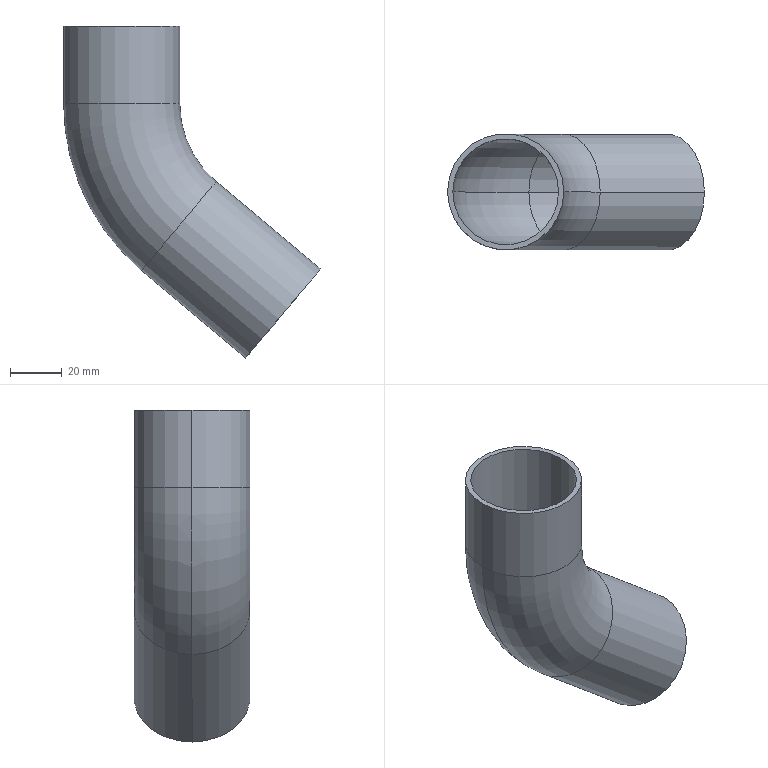Part | SolidWorks | features Shell 1, Sweep 1 | 1 solid | 14 faces | box 99.465 x 45 x 128.591 mm | volume 36956 mm3 | cylinder 8 | torus 4 | plane 2 | commonest cylinder face diameters 41 x4 45 x4
STEP:
#1=CARTESIAN_POINT('',(20.5,0.,-29.999));
#2=VERTEX_POINT('',#1);
#3=CARTESIAN_POINT('',(-20.5,0.,-29.999));
#4=VERTEX_POINT('',#3);
#5=CARTESIAN_POINT('',(0.,0.,-29.999));
#6=DIRECTION('',(0.,0.,1.));
#7=DIRECTION('',(1.,0.,0.));
#8=AXIS2_PLACEMENT_3D('',#5,#6,#7);
#9=CIRCLE('',#8,20.5);
#10=EDGE_CURVE('',#2,#4,#9,.T.);
#11=ORIENTED_EDGE('',*,*,#10,.T.);
#12=CARTESIAN_POINT('',(8.97,0.,-93.198));
#13=VERTEX_POINT('',#12);
#14=CARTESIAN_POINT('',(62.,0.,-29.999));
#15=DIRECTION('',(0.,-1.,0.));
#16=DIRECTION('',(0.,0.,-1.));
#17=AXIS2_PLACEMENT_3D('',#14,#15,#16);
#18=CIRCLE('',#17,82.5);
#19=EDGE_CURVE('',#4,#13,#18,.T.);
#20=ORIENTED_EDGE('',*,*,#19,.T.);
#21=CARTESIAN_POINT('',(35.324,0.,-61.79));
#22=VERTEX_POINT('',#21);
#23=CARTESIAN_POINT('',(22.147,0.,-77.494));
#24=DIRECTION('',(-0.766,0.,0.6428));
#25=DIRECTION('',(0.6428,0.,0.766));
#26=AXIS2_PLACEMENT_3D('',#23,#24,#25);
#27=CIRCLE('',#26,20.5);
#28=EDGE_CURVE('',#22,#13,#27,.T.);
#29=ORIENTED_EDGE('',*,*,#28,.F.);
#30=CARTESIAN_POINT('',(62.,0.,-29.999));
#31=DIRECTION('',(0.,-1.,0.));
#32=DIRECTION('',(0.,0.,-1.));
#33=AXIS2_PLACEMENT_3D('',#30,#31,#32);
#34=CIRCLE('',#33,41.5);
#35=EDGE_CURVE('',#2,#22,#34,.T.);
#36=ORIENTED_EDGE('',*,*,#35,.F.);
#37=EDGE_LOOP('',(#11,#20,#29,#36));
#38=FACE_OUTER_BOUND('',#37,.T.);
#39=CARTESIAN_POINT('',(62.,0.,-29.999));
#40=DIRECTION('',(0.,-1.,0.));
#41=DIRECTION('',(0.,0.,-1.));
#42=AXIS2_PLACEMENT_3D('',#39,#40,#41);
#43=TOROIDAL_SURFACE('',#42,62.,20.5);
#44=ADVANCED_FACE('',(#38),#43,.F.);
#45=CARTESIAN_POINT('',(-22.5,0.,-29.999));
#46=VERTEX_POINT('',#45);
#47=CARTESIAN_POINT('',(22.5,0.,-29.999));
#48=VERTEX_POINT('',#47);
#49=CARTESIAN_POINT('',(0.,0.,-29.999));
#50=DIRECTION('',(0.,0.,1.));
#51=DIRECTION('',(1.,0.,0.));
#52=AXIS2_PLACEMENT_3D('',#49,#50,#51);
#53=CIRCLE('',#52,22.5);
#54=EDGE_CURVE('',#46,#48,#53,.T.);
#55=ORIENTED_EDGE('',*,*,#54,.F.);
#56=CARTESIAN_POINT('',(7.684,0.,-94.73));
#57=VERTEX_POINT('',#56);
#58=CARTESIAN_POINT('',(62.,0.,-29.999));
#59=DIRECTION('',(0.,-1.,0.));
#60=DIRECTION('',(0.,0.,-1.));
#61=AXIS2_PLACEMENT_3D('',#58,#59,#60);
#62=CIRCLE('',#61,84.5);
#63=EDGE_CURVE('',#46,#57,#62,.T.);
#64=ORIENTED_EDGE('',*,*,#63,.T.);
#65=CARTESIAN_POINT('',(36.61,0.,-60.258));
#66=VERTEX_POINT('',#65);
#67=CARTESIAN_POINT('',(22.147,0.,-77.494));
#68=DIRECTION('',(-0.766,0.,0.6428));
#69=DIRECTION('',(0.6428,0.,0.766));
#70=AXIS2_PLACEMENT_3D('',#67,#68,#69);
#71=CIRCLE('',#70,22.5);
#72=EDGE_CURVE('',#57,#66,#71,.T.);
#73=ORIENTED_EDGE('',*,*,#72,.T.);
#74=CARTESIAN_POINT('',(62.,0.,-29.999));
#75=DIRECTION('',(0.,-1.,0.));
#76=DIRECTION('',(0.,0.,-1.));
#77=AXIS2_PLACEMENT_3D('',#74,#75,#76);
#78=CIRCLE('',#77,39.5);
#79=EDGE_CURVE('',#48,#66,#78,.T.);
#80=ORIENTED_EDGE('',*,*,#79,.F.);
#81=EDGE_LOOP('',(#55,#64,#73,#80));
#82=FACE_OUTER_BOUND('',#81,.T.);
#83=CARTESIAN_POINT('',(62.,0.,-29.999));
#84=DIRECTION('',(0.,-1.,0.));
#85=DIRECTION('',(0.,0.,-1.));
#86=AXIS2_PLACEMENT_3D('',#83,#84,#85);
#87=TOROIDAL_SURFACE('',#86,62.,22.5);
#88=ADVANCED_FACE('',(#82),#87,.T.);
#89=CARTESIAN_POINT('',(0.,0.,-29.999));
#90=DIRECTION('',(0.,0.,1.));
#91=DIRECTION('',(1.,0.,0.));
#92=AXIS2_PLACEMENT_3D('',#89,#90,#91);
#93=CIRCLE('',#92,20.5);
#94=EDGE_CURVE('',#4,#2,#93,.T.);
#95=ORIENTED_EDGE('',*,*,#94,.F.);
#96=CARTESIAN_POINT('',(-20.5,0.,0.));
#97=VERTEX_POINT('',#96);
#98=CARTESIAN_POINT('',(-20.5,0.,-29.999));
#99=DIRECTION('',(0.,0.,1.));
#100=VECTOR('',#99,1000.);
#101=LINE('',#98,#100);
#102=EDGE_CURVE('',#4,#97,#101,.T.);
#103=ORIENTED_EDGE('',*,*,#102,.T.);
#104=CARTESIAN_POINT('',(20.5,0.,0.));
#105=VERTEX_POINT('',#104);
#106=CARTESIAN_POINT('',(0.,0.,0.));
#107=DIRECTION('',(0.,0.,1.));
#108=DIRECTION('',(1.,0.,0.));
#109=AXIS2_PLACEMENT_3D('',#106,#107,#108);
#110=CIRCLE('',#109,20.5);
#111=EDGE_CURVE('',#97,#105,#110,.T.);
#112=ORIENTED_EDGE('',*,*,#111,.T.);
#113=CARTESIAN_POINT('',(20.5,0.,-29.999));
#114=DIRECTION('',(0.,0.,1.));
#115=VECTOR('',#114,1000.);
#116=LINE('',#113,#115);
#117=EDGE_CURVE('',#2,#105,#116,.T.);
#118=ORIENTED_EDGE('',*,*,#117,.F.);
#119=EDGE_LOOP('',(#95,#103,#112,#118));
#120=FACE_OUTER_BOUND('',#119,.T.);
#121=CARTESIAN_POINT('',(0.,0.,-29.999));
#122=DIRECTION('',(0.,0.,1.));
#123=DIRECTION('',(1.,0.,0.));
#124=AXIS2_PLACEMENT_3D('',#121,#122,#123);
#125=CYLINDRICAL_SURFACE('',#124,20.5);
#126=ADVANCED_FACE('',(#120),#125,.F.);
#127=CARTESIAN_POINT('',(22.147,0.,-77.494));
#128=DIRECTION('',(-0.766,0.,0.6428));
#129=DIRECTION('',(0.6428,0.,0.766));
#130=AXIS2_PLACEMENT_3D('',#127,#128,#129);
#131=CIRCLE('',#130,20.5);
#132=EDGE_CURVE('',#13,#22,#131,.T.);
#133=ORIENTED_EDGE('',*,*,#132,.T.);
#134=CARTESIAN_POINT('',(75.679,0.,-95.652));
#135=VERTEX_POINT('',#134);
#136=CARTESIAN_POINT('',(35.324,0.,-61.79));
#137=DIRECTION('',(0.766,0.,-0.6428));
#138=VECTOR('',#137,1000.);
#139=LINE('',#136,#138);
#140=EDGE_CURVE('',#22,#135,#139,.T.);
#141=ORIENTED_EDGE('',*,*,#140,.T.);
#142=CARTESIAN_POINT('',(49.325,0.,-127.059));
#143=VERTEX_POINT('',#142);
#144=CARTESIAN_POINT('',(62.502,0.,-111.355));
#145=DIRECTION('',(-0.766,0.,0.6428));
#146=DIRECTION('',(0.6428,0.,0.766));
#147=AXIS2_PLACEMENT_3D('',#144,#145,#146);
#148=CIRCLE('',#147,20.5);
#149=EDGE_CURVE('',#143,#135,#148,.T.);
#150=ORIENTED_EDGE('',*,*,#149,.F.);
#151=CARTESIAN_POINT('',(8.97,0.,-93.198));
#152=DIRECTION('',(0.766,0.,-0.6428));
#153=VECTOR('',#152,1000.);
#154=LINE('',#151,#153);
#155=EDGE_CURVE('',#13,#143,#154,.T.);
#156=ORIENTED_EDGE('',*,*,#155,.F.);
#157=EDGE_LOOP('',(#133,#141,#150,#156));
#158=FACE_OUTER_BOUND('',#157,.T.);
#159=CARTESIAN_POINT('',(22.147,0.,-77.494));
#160=DIRECTION('',(0.766,0.,-0.6428));
#161=DIRECTION('',(-0.6428,0.,-0.766));
#162=AXIS2_PLACEMENT_3D('',#159,#160,#161);
#163=CYLINDRICAL_SURFACE('',#162,20.5);
#164=ADVANCED_FACE('',(#158),#163,.F.);
#165=CARTESIAN_POINT('',(0.,0.,-29.999));
#166=DIRECTION('',(0.,0.,1.));
#167=DIRECTION('',(1.,0.,0.));
#168=AXIS2_PLACEMENT_3D('',#165,#166,#167);
#169=CIRCLE('',#168,22.5);
#170=EDGE_CURVE('',#48,#46,#169,.T.);
#171=ORIENTED_EDGE('',*,*,#170,.T.);
#172=CARTESIAN_POINT('',(-22.5,0.,0.));
#173=VERTEX_POINT('',#172);
#174=CARTESIAN_POINT('',(-22.5,0.,-29.999));
#175=DIRECTION('',(0.,0.,1.));
#176=VECTOR('',#175,1000.);
#177=LINE('',#174,#176);
#178=EDGE_CURVE('',#46,#173,#177,.T.);
#179=ORIENTED_EDGE('',*,*,#178,.T.);
#180=CARTESIAN_POINT('',(22.5,0.,0.));
#181=VERTEX_POINT('',#180);
#182=CARTESIAN_POINT('',(0.,0.,0.));
#183=DIRECTION('',(0.,0.,1.));
#184=DIRECTION('',(1.,0.,0.));
#185=AXIS2_PLACEMENT_3D('',#182,#183,#184);
#186=CIRCLE('',#185,22.5);
#187=EDGE_CURVE('',#181,#173,#186,.T.);
#188=ORIENTED_EDGE('',*,*,#187,.F.);
#189=CARTESIAN_POINT('',(22.5,0.,-29.999));
#190=DIRECTION('',(0.,0.,1.));
#191=VECTOR('',#190,1000.);
#192=LINE('',#189,#191);
#193=EDGE_CURVE('',#48,#181,#192,.T.);
#194=ORIENTED_EDGE('',*,*,#193,.F.);
#195=EDGE_LOOP('',(#171,#179,#188,#194));
#196=FACE_OUTER_BOUND('',#195,.T.);
#197=CARTESIAN_POINT('',(0.,0.,-29.999));
#198=DIRECTION('',(0.,0.,1.));
#199=DIRECTION('',(1.,0.,0.));
#200=AXIS2_PLACEMENT_3D('',#197,#198,#199);
#201=CYLINDRICAL_SURFACE('',#200,22.5);
#202=ADVANCED_FACE('',(#196),#201,.T.);
#203=CARTESIAN_POINT('',(22.147,0.,-77.494));
#204=DIRECTION('',(-0.766,0.,0.6428));
#205=DIRECTION('',(0.6428,0.,0.766));
#206=AXIS2_PLACEMENT_3D('',#203,#204,#205);
#207=CIRCLE('',#206,22.5);
#208=EDGE_CURVE('',#66,#57,#207,.T.);
#209=ORIENTED_EDGE('',*,*,#208,.F.);
#210=CARTESIAN_POINT('',(76.965,0.,-94.119));
#211=VERTEX_POINT('',#210);
#212=CARTESIAN_POINT('',(36.61,0.,-60.258));
#213=DIRECTION('',(0.766,0.,-0.6428));
#214=VECTOR('',#213,1000.);
#215=LINE('',#212,#214);
#216=EDGE_CURVE('',#66,#211,#215,.T.);
#217=ORIENTED_EDGE('',*,*,#216,.T.);
#218=CARTESIAN_POINT('',(48.039,0.,-128.591));
#219=VERTEX_POINT('',#218);
#220=CARTESIAN_POINT('',(62.502,0.,-111.355));
#221=DIRECTION('',(-0.766,0.,0.6428));
#222=DIRECTION('',(0.6428,0.,0.766));
#223=AXIS2_PLACEMENT_3D('',#220,#221,#222);
#224=CIRCLE('',#223,22.5);
#225=EDGE_CURVE('',#211,#219,#224,.T.);
#226=ORIENTED_EDGE('',*,*,#225,.T.);
#227=CARTESIAN_POINT('',(7.684,0.,-94.73));
#228=DIRECTION('',(0.766,0.,-0.6428));
#229=VECTOR('',#228,1000.);
#230=LINE('',#227,#229);
#231=EDGE_CURVE('',#57,#219,#230,.T.);
#232=ORIENTED_EDGE('',*,*,#231,.F.);
#233=EDGE_LOOP('',(#209,#217,#226,#232));
#234=FACE_OUTER_BOUND('',#233,.T.);
#235=CARTESIAN_POINT('',(22.147,0.,-77.494));
#236=DIRECTION('',(0.766,0.,-0.6428));
#237=DIRECTION('',(-0.6428,0.,-0.766));
#238=AXIS2_PLACEMENT_3D('',#235,#236,#237);
#239=CYLINDRICAL_SURFACE('',#238,22.5);
#240=ADVANCED_FACE('',(#234),#239,.T.);
#241=ORIENTED_EDGE('',*,*,#216,.F.);
#242=ORIENTED_EDGE('',*,*,#72,.F.);
#243=ORIENTED_EDGE('',*,*,#231,.T.);
#244=CARTESIAN_POINT('',(62.502,0.,-111.355));
#245=DIRECTION('',(-0.766,0.,0.6428));
#246=DIRECTION('',(0.6428,0.,0.766));
#247=AXIS2_PLACEMENT_3D('',#244,#245,#246);
#248=CIRCLE('',#247,22.5);
#249=EDGE_CURVE('',#219,#211,#248,.T.);
#250=ORIENTED_EDGE('',*,*,#249,.T.);
#251=EDGE_LOOP('',(#241,#242,#243,#250));
#252=FACE_OUTER_BOUND('',#251,.T.);
#253=CARTESIAN_POINT('',(22.147,0.,-77.494));
#254=DIRECTION('',(0.766,0.,-0.6428));
#255=DIRECTION('',(-0.6428,0.,-0.766));
#256=AXIS2_PLACEMENT_3D('',#253,#254,#255);
#257=CYLINDRICAL_SURFACE('',#256,22.5);
#258=ADVANCED_FACE('',(#252),#257,.T.);
#259=ORIENTED_EDGE('',*,*,#63,.F.);
#260=ORIENTED_EDGE('',*,*,#170,.F.);
#261=ORIENTED_EDGE('',*,*,#79,.T.);
#262=ORIENTED_EDGE('',*,*,#208,.T.);
#263=EDGE_LOOP('',(#259,#260,#261,#262));
#264=FACE_OUTER_BOUND('',#263,.T.);
#265=CARTESIAN_POINT('',(62.,0.,-29.999));
#266=DIRECTION('',(0.,-1.,0.));
#267=DIRECTION('',(0.,0.,-1.));
#268=AXIS2_PLACEMENT_3D('',#265,#266,#267);
#269=TOROIDAL_SURFACE('',#268,62.,22.5);
#270=ADVANCED_FACE('',(#264),#269,.T.);
#271=ORIENTED_EDGE('',*,*,#178,.F.);
#272=ORIENTED_EDGE('',*,*,#54,.T.);
#273=ORIENTED_EDGE('',*,*,#193,.T.);
#274=CARTESIAN_POINT('',(0.,0.,0.));
#275=DIRECTION('',(0.,0.,1.));
#276=DIRECTION('',(1.,0.,0.));
#277=AXIS2_PLACEMENT_3D('',#274,#275,#276);
#278=CIRCLE('',#277,22.5);
#279=EDGE_CURVE('',#173,#181,#278,.T.);
#280=ORIENTED_EDGE('',*,*,#279,.F.);
#281=EDGE_LOOP('',(#271,#272,#273,#280));
#282=FACE_OUTER_BOUND('',#281,.T.);
#283=CARTESIAN_POINT('',(0.,0.,-29.999));
#284=DIRECTION('',(0.,0.,1.));
#285=DIRECTION('',(1.,0.,0.));
#286=AXIS2_PLACEMENT_3D('',#283,#284,#285);
#287=CYLINDRICAL_SURFACE('',#286,22.5);
#288=ADVANCED_FACE('',(#282),#287,.T.);
#289=ORIENTED_EDGE('',*,*,#149,.T.);
#290=CARTESIAN_POINT('',(62.502,0.,-111.355));
#291=DIRECTION('',(-0.766,0.,0.6428));
#292=DIRECTION('',(0.6428,0.,0.766));
#293=AXIS2_PLACEMENT_3D('',#290,#291,#292);
#294=CIRCLE('',#293,20.5);
#295=EDGE_CURVE('',#135,#143,#294,.T.);
#296=ORIENTED_EDGE('',*,*,#295,.T.);
#297=EDGE_LOOP('',(#289,#296));
#298=FACE_BOUND('',#297,.T.);
#299=ORIENTED_EDGE('',*,*,#249,.F.);
#300=ORIENTED_EDGE('',*,*,#225,.F.);
#301=EDGE_LOOP('',(#299,#300));
#302=FACE_OUTER_BOUND('',#301,.T.);
#303=CARTESIAN_POINT('',(62.502,0.,-111.355));
#304=DIRECTION('',(-0.766,0.,0.6428));
#305=DIRECTION('',(0.6428,0.,0.766));
#306=AXIS2_PLACEMENT_3D('',#303,#304,#305);
#307=PLANE('',#306);
#308=ADVANCED_FACE('',(#298,#302),#307,.F.);
#309=CARTESIAN_POINT('',(0.,0.,0.));
#310=DIRECTION('',(0.,0.,1.));
#311=DIRECTION('',(1.,0.,0.));
#312=AXIS2_PLACEMENT_3D('',#309,#310,#311);
#313=CIRCLE('',#312,20.5);
#314=EDGE_CURVE('',#105,#97,#313,.T.);
#315=ORIENTED_EDGE('',*,*,#314,.F.);
#316=ORIENTED_EDGE('',*,*,#111,.F.);
#317=EDGE_LOOP('',(#315,#316));
#318=FACE_BOUND('',#317,.T.);
#319=ORIENTED_EDGE('',*,*,#187,.T.);
#320=ORIENTED_EDGE('',*,*,#279,.T.);
#321=EDGE_LOOP('',(#319,#320));
#322=FACE_OUTER_BOUND('',#321,.T.);
#323=CARTESIAN_POINT('',(0.,0.,0.));
#324=DIRECTION('',(0.,0.,1.));
#325=DIRECTION('',(1.,0.,0.));
#326=AXIS2_PLACEMENT_3D('',#323,#324,#325);
#327=PLANE('',#326);
#328=ADVANCED_FACE('',(#318,#322),#327,.T.);
#329=ORIENTED_EDGE('',*,*,#140,.F.);
#330=ORIENTED_EDGE('',*,*,#28,.T.);
#331=ORIENTED_EDGE('',*,*,#155,.T.);
#332=ORIENTED_EDGE('',*,*,#295,.F.);
#333=EDGE_LOOP('',(#329,#330,#331,#332));
#334=FACE_OUTER_BOUND('',#333,.T.);
#335=CARTESIAN_POINT('',(22.147,0.,-77.494));
#336=DIRECTION('',(0.766,0.,-0.6428));
#337=DIRECTION('',(-0.6428,0.,-0.766));
#338=AXIS2_PLACEMENT_3D('',#335,#336,#337);
#339=CYLINDRICAL_SURFACE('',#338,20.5);
#340=ADVANCED_FACE('',(#334),#339,.F.);
#341=ORIENTED_EDGE('',*,*,#19,.F.);
#342=ORIENTED_EDGE('',*,*,#94,.T.);
#343=ORIENTED_EDGE('',*,*,#35,.T.);
#344=ORIENTED_EDGE('',*,*,#132,.F.);
#345=EDGE_LOOP('',(#341,#342,#343,#344));
#346=FACE_OUTER_BOUND('',#345,.T.);
#347=CARTESIAN_POINT('',(62.,0.,-29.999));
#348=DIRECTION('',(0.,-1.,0.));
#349=DIRECTION('',(0.,0.,-1.));
#350=AXIS2_PLACEMENT_3D('',#347,#348,#349);
#351=TOROIDAL_SURFACE('',#350,62.,20.5);
#352=ADVANCED_FACE('',(#346),#351,.F.);
#353=ORIENTED_EDGE('',*,*,#102,.F.);
#354=ORIENTED_EDGE('',*,*,#10,.F.);
#355=ORIENTED_EDGE('',*,*,#117,.T.);
#356=ORIENTED_EDGE('',*,*,#314,.T.);
#357=EDGE_LOOP('',(#353,#354,#355,#356));
#358=FACE_OUTER_BOUND('',#357,.T.);
#359=CARTESIAN_POINT('',(0.,0.,-29.999));
#360=DIRECTION('',(0.,0.,1.));
#361=DIRECTION('',(1.,0.,0.));
#362=AXIS2_PLACEMENT_3D('',#359,#360,#361);
#363=CYLINDRICAL_SURFACE('',#362,20.5);
#364=ADVANCED_FACE('',(#358),#363,.F.);
#365=CLOSED_SHELL('',(#44,#88,#126,#164,#202,#240,#258,#270,#288,#308,#328,#340,#352,#364));
#366=MANIFOLD_SOLID_BREP('',#365);
#367=CARTESIAN_POINT('',(0.,0.,0.));
#368=DIRECTION('',(0.,0.,1.));
#369=DIRECTION('',(1.,0.,0.));
#370=AXIS2_PLACEMENT_3D('',#367,#368,#369);
#371=(LENGTH_UNIT()NAMED_UNIT(*)SI_UNIT(.MILLI.,.METRE.));
#372=UNCERTAINTY_MEASURE_WITH_UNIT(LENGTH_MEASURE(0.00001),#371,'','');
#373=(NAMED_UNIT(*)PLANE_ANGLE_UNIT()SI_UNIT($,.RADIAN.));
#374=(NAMED_UNIT(*)SI_UNIT($,.STERADIAN.)SOLID_ANGLE_UNIT());
#375=(GEOMETRIC_REPRESENTATION_CONTEXT(3)GLOBAL_UNCERTAINTY_ASSIGNED_CONTEXT((#372))GLOBAL_UNIT_ASSIGNED_CONTEXT((#371,#373,#374))REPRESENTATION_CONTEXT('',''));
#376=ADVANCED_BREP_SHAPE_REPRESENTATION('',(#366,#370),#375);